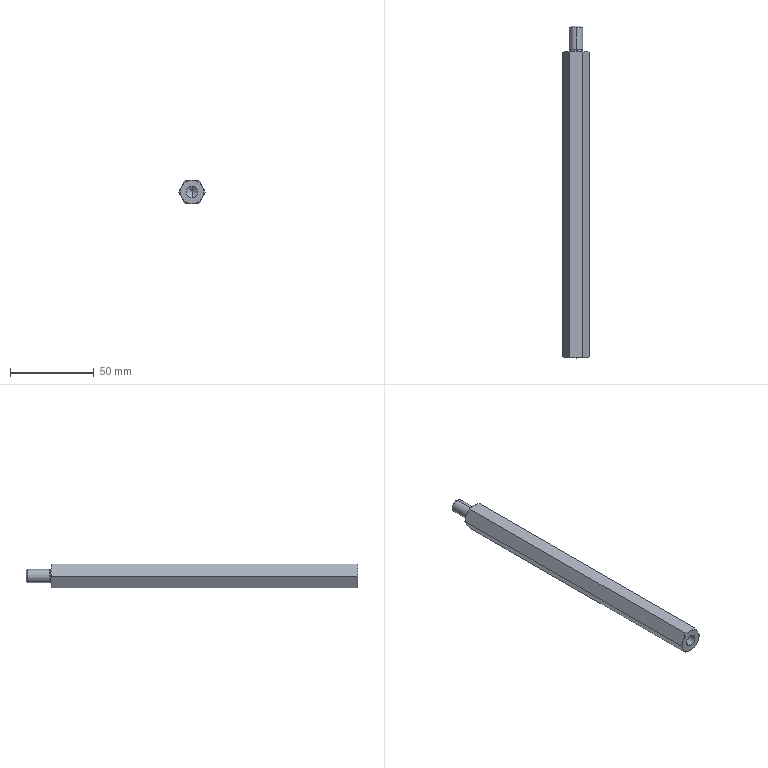Part | STEP file | 0229_204_Stud | 1 solid | 33 faces | box 16.166 x 198.5 x 14 mm | volume 31042 mm3 | cone 16 | plane 9 | torus 4 | cylinder 4 | commonest cylinder face diameters 6.8 x2 8 x2